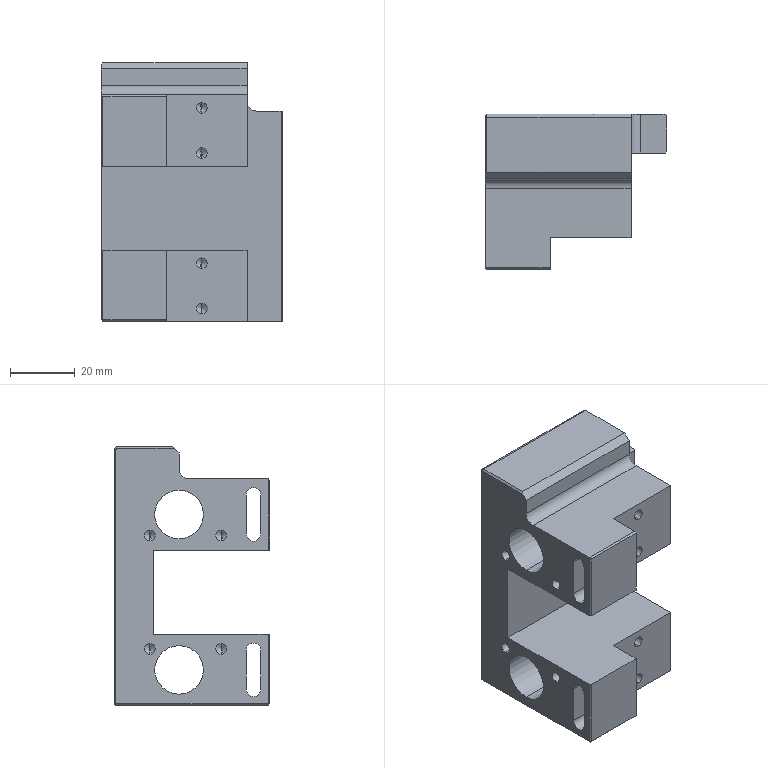Part | SolidWorks | features HoleWzd 9, ICE 9, Chamfer 3, Fillet 2, CutThin 1, Extrusion 1, LPattern 1 | 1 solid | 178 faces | box 56 x 48 x 80 mm | volume 94389 mm3 | cylinder 93 | cone 45 | plane 40 | commonest cylinder face diameters 1 x48 3.3 x28 4.5 x6 4.2 x4 15 x4 6 x2